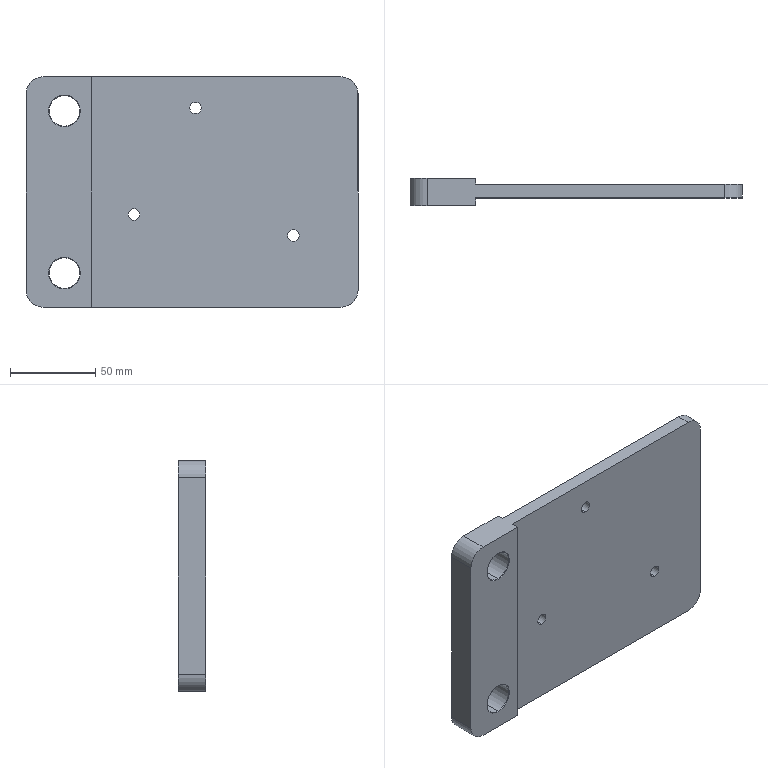Part | SolidWorks | features ICE 4, Chamfer 2, Fillet 1, FlatPattern 1, HoleWzd 1, SMBaseFlange 1, SheetMetal 1 | 1 solid | 39 faces | box 194.5 x 16 x 135 mm | volume 211709 mm3 | cylinder 16 | plane 11 | cone 10 | torus 2 | commonest cylinder face diameters 6.8 x6 18 x4 20 x4 83 x2
STEP:
#1=CARTESIAN_POINT('',(22.5,-0.3,11.));
#2=VERTEX_POINT('',#1);
#3=CARTESIAN_POINT('',(22.5,-0.3,29.));
#4=VERTEX_POINT('',#3);
#5=CARTESIAN_POINT('',(22.5,-0.3,20.));
#6=DIRECTION('',(0.,1.,0.));
#7=DIRECTION('',(0.,0.,-1.));
#8=AXIS2_PLACEMENT_3D('',#5,#6,#7);
#9=CIRCLE('',#8,9.);
#10=EDGE_CURVE('',#2,#4,#9,.T.);
#11=ORIENTED_EDGE('',*,*,#10,.F.);
#12=CARTESIAN_POINT('',(22.5,0.,10.7));
#13=VERTEX_POINT('',#12);
#14=CARTESIAN_POINT('',(22.5,-0.3,11.));
#15=DIRECTION('',(0.,0.7071,-0.7071));
#16=VECTOR('',#15,1000.);
#17=LINE('',#14,#16);
#18=EDGE_CURVE('',#2,#13,#17,.T.);
#19=ORIENTED_EDGE('',*,*,#18,.T.);
#20=CARTESIAN_POINT('',(22.5,0.,29.3));
#21=VERTEX_POINT('',#20);
#22=CARTESIAN_POINT('',(22.5,0.,20.));
#23=DIRECTION('',(0.,-1.,0.));
#24=DIRECTION('',(0.,0.,-1.));
#25=AXIS2_PLACEMENT_3D('',#22,#23,#24);
#26=CIRCLE('',#25,9.3);
#27=EDGE_CURVE('',#21,#13,#26,.T.);
#28=ORIENTED_EDGE('',*,*,#27,.F.);
#29=CARTESIAN_POINT('',(22.5,-0.3,29.));
#30=DIRECTION('',(0.,0.7071,0.7071));
#31=VECTOR('',#30,1000.);
#32=LINE('',#29,#31);
#33=EDGE_CURVE('',#4,#21,#32,.T.);
#34=ORIENTED_EDGE('',*,*,#33,.F.);
#35=EDGE_LOOP('',(#11,#19,#28,#34));
#36=FACE_OUTER_BOUND('',#35,.T.);
#37=CARTESIAN_POINT('',(22.5,-0.3,20.));
#38=DIRECTION('',(0.,1.,0.));
#39=DIRECTION('',(0.,0.,1.));
#40=AXIS2_PLACEMENT_3D('',#37,#38,#39);
#41=CONICAL_SURFACE('',#40,9.,0.7854);
#42=ADVANCED_FACE('',(#36),#41,.F.);
#43=CARTESIAN_POINT('',(22.5,-15.7,29.));
#44=VERTEX_POINT('',#43);
#45=CARTESIAN_POINT('',(22.5,-15.7,11.));
#46=VERTEX_POINT('',#45);
#47=CARTESIAN_POINT('',(22.5,-15.7,20.));
#48=DIRECTION('',(0.,-1.,0.));
#49=DIRECTION('',(0.,0.,-1.));
#50=AXIS2_PLACEMENT_3D('',#47,#48,#49);
#51=CIRCLE('',#50,9.);
#52=EDGE_CURVE('',#44,#46,#51,.T.);
#53=ORIENTED_EDGE('',*,*,#52,.F.);
#54=CARTESIAN_POINT('',(22.5,-16.,29.3));
#55=VERTEX_POINT('',#54);
#56=CARTESIAN_POINT('',(22.5,-16.,29.3));
#57=DIRECTION('',(0.,-0.7071,0.7071));
#58=VECTOR('',#57,1000.);
#59=LINE('',#56,#58);
#60=EDGE_CURVE('',#44,#55,#59,.T.);
#61=ORIENTED_EDGE('',*,*,#60,.T.);
#62=CARTESIAN_POINT('',(22.5,-16.,10.7));
#63=VERTEX_POINT('',#62);
#64=CARTESIAN_POINT('',(22.5,-16.,20.));
#65=DIRECTION('',(0.,1.,0.));
#66=DIRECTION('',(0.,0.,-1.));
#67=AXIS2_PLACEMENT_3D('',#64,#65,#66);
#68=CIRCLE('',#67,9.3);
#69=EDGE_CURVE('',#63,#55,#68,.T.);
#70=ORIENTED_EDGE('',*,*,#69,.F.);
#71=CARTESIAN_POINT('',(22.5,-16.,10.7));
#72=DIRECTION('',(0.,-0.7071,-0.7071));
#73=VECTOR('',#72,1000.);
#74=LINE('',#71,#73);
#75=EDGE_CURVE('',#46,#63,#74,.T.);
#76=ORIENTED_EDGE('',*,*,#75,.F.);
#77=EDGE_LOOP('',(#53,#61,#70,#76));
#78=FACE_OUTER_BOUND('',#77,.T.);
#79=CARTESIAN_POINT('',(22.5,-16.,20.));
#80=DIRECTION('',(0.,-1.,0.));
#81=DIRECTION('',(0.,0.,-1.));
#82=AXIS2_PLACEMENT_3D('',#79,#80,#81);
#83=CONICAL_SURFACE('',#82,9.3,0.7854);
#84=ADVANCED_FACE('',(#78),#83,.F.);
#85=CARTESIAN_POINT('',(22.5,-15.7,124.));
#86=VERTEX_POINT('',#85);
#87=CARTESIAN_POINT('',(22.5,-15.7,106.));
#88=VERTEX_POINT('',#87);
#89=CARTESIAN_POINT('',(22.5,-15.7,115.));
#90=DIRECTION('',(0.,-1.,0.));
#91=DIRECTION('',(0.,0.,-1.));
#92=AXIS2_PLACEMENT_3D('',#89,#90,#91);
#93=CIRCLE('',#92,9.);
#94=EDGE_CURVE('',#86,#88,#93,.T.);
#95=ORIENTED_EDGE('',*,*,#94,.F.);
#96=CARTESIAN_POINT('',(22.5,-16.,124.3));
#97=VERTEX_POINT('',#96);
#98=CARTESIAN_POINT('',(22.5,-16.,124.3));
#99=DIRECTION('',(0.,-0.7071,0.7071));
#100=VECTOR('',#99,1000.);
#101=LINE('',#98,#100);
#102=EDGE_CURVE('',#86,#97,#101,.T.);
#103=ORIENTED_EDGE('',*,*,#102,.T.);
#104=CARTESIAN_POINT('',(22.5,-16.,105.7));
#105=VERTEX_POINT('',#104);
#106=CARTESIAN_POINT('',(22.5,-16.,115.));
#107=DIRECTION('',(0.,1.,0.));
#108=DIRECTION('',(0.,0.,-1.));
#109=AXIS2_PLACEMENT_3D('',#106,#107,#108);
#110=CIRCLE('',#109,9.3);
#111=EDGE_CURVE('',#105,#97,#110,.T.);
#112=ORIENTED_EDGE('',*,*,#111,.F.);
#113=CARTESIAN_POINT('',(22.5,-16.,105.7));
#114=DIRECTION('',(0.,-0.7071,-0.7071));
#115=VECTOR('',#114,1000.);
#116=LINE('',#113,#115);
#117=EDGE_CURVE('',#88,#105,#116,.T.);
#118=ORIENTED_EDGE('',*,*,#117,.F.);
#119=EDGE_LOOP('',(#95,#103,#112,#118));
#120=FACE_OUTER_BOUND('',#119,.T.);
#121=CARTESIAN_POINT('',(22.5,-16.,115.));
#122=DIRECTION('',(0.,-1.,0.));
#123=DIRECTION('',(0.,0.,-1.));
#124=AXIS2_PLACEMENT_3D('',#121,#122,#123);
#125=CONICAL_SURFACE('',#124,9.3,0.7854);
#126=ADVANCED_FACE('',(#120),#125,.F.);
#127=CARTESIAN_POINT('',(22.5,-0.3,106.));
#128=VERTEX_POINT('',#127);
#129=CARTESIAN_POINT('',(22.5,-0.3,124.));
#130=VERTEX_POINT('',#129);
#131=CARTESIAN_POINT('',(22.5,-0.3,115.));
#132=DIRECTION('',(0.,1.,0.));
#133=DIRECTION('',(0.,0.,-1.));
#134=AXIS2_PLACEMENT_3D('',#131,#132,#133);
#135=CIRCLE('',#134,9.);
#136=EDGE_CURVE('',#128,#130,#135,.T.);
#137=ORIENTED_EDGE('',*,*,#136,.F.);
#138=CARTESIAN_POINT('',(22.5,0.,105.7));
#139=VERTEX_POINT('',#138);
#140=CARTESIAN_POINT('',(22.5,-0.3,106.));
#141=DIRECTION('',(0.,0.7071,-0.7071));
#142=VECTOR('',#141,1000.);
#143=LINE('',#140,#142);
#144=EDGE_CURVE('',#128,#139,#143,.T.);
#145=ORIENTED_EDGE('',*,*,#144,.T.);
#146=CARTESIAN_POINT('',(22.5,0.,124.3));
#147=VERTEX_POINT('',#146);
#148=CARTESIAN_POINT('',(22.5,0.,115.));
#149=DIRECTION('',(0.,-1.,0.));
#150=DIRECTION('',(0.,0.,-1.));
#151=AXIS2_PLACEMENT_3D('',#148,#149,#150);
#152=CIRCLE('',#151,9.3);
#153=EDGE_CURVE('',#147,#139,#152,.T.);
#154=ORIENTED_EDGE('',*,*,#153,.F.);
#155=CARTESIAN_POINT('',(22.5,-0.3,124.));
#156=DIRECTION('',(0.,0.7071,0.7071));
#157=VECTOR('',#156,1000.);
#158=LINE('',#155,#157);
#159=EDGE_CURVE('',#130,#147,#158,.T.);
#160=ORIENTED_EDGE('',*,*,#159,.F.);
#161=EDGE_LOOP('',(#137,#145,#154,#160));
#162=FACE_OUTER_BOUND('',#161,.T.);
#163=CARTESIAN_POINT('',(22.5,-0.3,115.));
#164=DIRECTION('',(0.,1.,0.));
#165=DIRECTION('',(0.,0.,1.));
#166=AXIS2_PLACEMENT_3D('',#163,#164,#165);
#167=CONICAL_SURFACE('',#166,9.,0.7854);
#168=ADVANCED_FACE('',(#162),#167,.F.);
#169=CARTESIAN_POINT('',(112.5,-4.5,26.));
#170=VERTEX_POINT('',#169);
#171=CARTESIAN_POINT('',(112.5,-4.5,109.));
#172=VERTEX_POINT('',#171);
#173=CARTESIAN_POINT('',(112.5,-4.5,67.5));
#174=DIRECTION('',(0.,1.,0.));
#175=DIRECTION('',(0.,0.,1.));
#176=AXIS2_PLACEMENT_3D('',#173,#174,#175);
#177=CIRCLE('',#176,41.5);
#178=EDGE_CURVE('',#170,#172,#177,.T.);
#179=ORIENTED_EDGE('',*,*,#178,.F.);
#180=CARTESIAN_POINT('',(112.5,-3.5,25.));
#181=VERTEX_POINT('',#180);
#182=CARTESIAN_POINT('',(112.5,-4.5,26.));
#183=DIRECTION('',(0.,0.7071,-0.7071));
#184=VECTOR('',#183,1000.);
#185=LINE('',#182,#184);
#186=EDGE_CURVE('',#170,#181,#185,.T.);
#187=ORIENTED_EDGE('',*,*,#186,.T.);
#188=CARTESIAN_POINT('',(112.5,-3.5,110.));
#189=VERTEX_POINT('',#188);
#190=CARTESIAN_POINT('',(112.5,-3.5,67.5));
#191=DIRECTION('',(0.,-1.,0.));
#192=DIRECTION('',(0.,0.,1.));
#193=AXIS2_PLACEMENT_3D('',#190,#191,#192);
#194=CIRCLE('',#193,42.5);
#195=EDGE_CURVE('',#189,#181,#194,.T.);
#196=ORIENTED_EDGE('',*,*,#195,.F.);
#197=CARTESIAN_POINT('',(112.5,-4.5,109.));
#198=DIRECTION('',(0.,0.7071,0.7071));
#199=VECTOR('',#198,1000.);
#200=LINE('',#197,#199);
#201=EDGE_CURVE('',#172,#189,#200,.T.);
#202=ORIENTED_EDGE('',*,*,#201,.F.);
#203=EDGE_LOOP('',(#179,#187,#196,#202));
#204=FACE_OUTER_BOUND('',#203,.T.);
#205=CARTESIAN_POINT('',(112.5,-4.5,67.5));
#206=DIRECTION('',(0.,1.,0.));
#207=DIRECTION('',(0.,0.,1.));
#208=AXIS2_PLACEMENT_3D('',#205,#206,#207);
#209=CONICAL_SURFACE('',#208,41.5,0.7854);
#210=ADVANCED_FACE('',(#204),#209,.F.);
#211=CARTESIAN_POINT('',(112.5,-9.,26.5));
#212=VERTEX_POINT('',#211);
#213=CARTESIAN_POINT('',(112.5,-9.,108.5));
#214=VERTEX_POINT('',#213);
#215=CARTESIAN_POINT('',(112.5,-9.,67.5));
#216=DIRECTION('',(0.,1.,0.));
#217=DIRECTION('',(0.,0.,1.));
#218=AXIS2_PLACEMENT_3D('',#215,#216,#217);
#219=CIRCLE('',#218,41.);
#220=EDGE_CURVE('',#212,#214,#219,.T.);
#221=ORIENTED_EDGE('',*,*,#220,.F.);
#222=CARTESIAN_POINT('',(112.5,-8.5,26.));
#223=VERTEX_POINT('',#222);
#224=CARTESIAN_POINT('',(112.5,-8.5,26.5));
#225=DIRECTION('',(1.,0.,0.));
#226=DIRECTION('',(0.,0.,-1.));
#227=AXIS2_PLACEMENT_3D('',#224,#225,#226);
#228=CIRCLE('',#227,0.5);
#229=EDGE_CURVE('',#212,#223,#228,.T.);
#230=ORIENTED_EDGE('',*,*,#229,.T.);
#231=CARTESIAN_POINT('',(112.5,-8.5,109.));
#232=VERTEX_POINT('',#231);
#233=CARTESIAN_POINT('',(112.5,-8.5,67.5));
#234=DIRECTION('',(0.,-1.,0.));
#235=DIRECTION('',(0.,0.,1.));
#236=AXIS2_PLACEMENT_3D('',#233,#234,#235);
#237=CIRCLE('',#236,41.5);
#238=EDGE_CURVE('',#232,#223,#237,.T.);
#239=ORIENTED_EDGE('',*,*,#238,.F.);
#240=CARTESIAN_POINT('',(112.5,-8.5,108.5));
#241=DIRECTION('',(-1.,0.,0.));
#242=DIRECTION('',(0.,0.,1.));
#243=AXIS2_PLACEMENT_3D('',#240,#241,#242);
#244=CIRCLE('',#243,0.5);
#245=EDGE_CURVE('',#214,#232,#244,.T.);
#246=ORIENTED_EDGE('',*,*,#245,.F.);
#247=EDGE_LOOP('',(#221,#230,#239,#246));
#248=FACE_OUTER_BOUND('',#247,.T.);
#249=CARTESIAN_POINT('',(112.5,-8.5,67.5));
#250=DIRECTION('',(0.,1.,0.));
#251=DIRECTION('',(0.,0.,1.));
#252=AXIS2_PLACEMENT_3D('',#249,#250,#251);
#253=TOROIDAL_SURFACE('',#252,41.,0.5);
#254=ADVANCED_FACE('',(#248),#253,.F.);
#255=CARTESIAN_POINT('',(63.238,-11.5,57.7));
#256=VERTEX_POINT('',#255);
#257=CARTESIAN_POINT('',(63.238,-11.5,50.9));
#258=VERTEX_POINT('',#257);
#259=CARTESIAN_POINT('',(63.238,-11.5,54.3));
#260=DIRECTION('',(0.,-1.,0.));
#261=DIRECTION('',(0.,0.,-1.));
#262=AXIS2_PLACEMENT_3D('',#259,#260,#261);
#263=CIRCLE('',#262,3.4);
#264=EDGE_CURVE('',#256,#258,#263,.T.);
#265=ORIENTED_EDGE('',*,*,#264,.T.);
#266=CARTESIAN_POINT('',(63.238,-3.5,50.9));
#267=VERTEX_POINT('',#266);
#268=CARTESIAN_POINT('',(63.238,-3.5,50.9));
#269=DIRECTION('',(0.,1.,0.));
#270=VECTOR('',#269,1000.);
#271=LINE('',#268,#270);
#272=EDGE_CURVE('',#258,#267,#271,.T.);
#273=ORIENTED_EDGE('',*,*,#272,.T.);
#274=CARTESIAN_POINT('',(63.238,-3.5,57.7));
#275=VERTEX_POINT('',#274);
#276=CARTESIAN_POINT('',(63.238,-3.5,54.3));
#277=DIRECTION('',(0.,1.,0.));
#278=DIRECTION('',(0.,0.,1.));
#279=AXIS2_PLACEMENT_3D('',#276,#277,#278);
#280=CIRCLE('',#279,3.4);
#281=EDGE_CURVE('',#267,#275,#280,.T.);
#282=ORIENTED_EDGE('',*,*,#281,.T.);
#283=CARTESIAN_POINT('',(63.238,-3.5,57.7));
#284=DIRECTION('',(0.,1.,0.));
#285=VECTOR('',#284,1000.);
#286=LINE('',#283,#285);
#287=EDGE_CURVE('',#256,#275,#286,.T.);
#288=ORIENTED_EDGE('',*,*,#287,.F.);
#289=EDGE_LOOP('',(#265,#273,#282,#288));
#290=FACE_OUTER_BOUND('',#289,.T.);
#291=CARTESIAN_POINT('',(63.238,-3.5,54.3));
#292=DIRECTION('',(0.,1.,0.));
#293=DIRECTION('',(0.,0.,1.));
#294=AXIS2_PLACEMENT_3D('',#291,#292,#293);
#295=CYLINDRICAL_SURFACE('',#294,3.4);
#296=ADVANCED_FACE('',(#290),#295,.F.);
#297=CARTESIAN_POINT('',(156.667,-11.5,45.4));
#298=VERTEX_POINT('',#297);
#299=CARTESIAN_POINT('',(156.667,-11.5,38.6));
#300=VERTEX_POINT('',#299);
#301=CARTESIAN_POINT('',(156.667,-11.5,42.));
#302=DIRECTION('',(0.,-1.,0.));
#303=DIRECTION('',(0.,0.,-1.));
#304=AXIS2_PLACEMENT_3D('',#301,#302,#303);
#305=CIRCLE('',#304,3.4);
#306=EDGE_CURVE('',#298,#300,#305,.T.);
#307=ORIENTED_EDGE('',*,*,#306,.T.);
#308=CARTESIAN_POINT('',(156.667,-3.5,38.6));
#309=VERTEX_POINT('',#308);
#310=CARTESIAN_POINT('',(156.667,-3.5,38.6));
#311=DIRECTION('',(0.,1.,0.));
#312=VECTOR('',#311,1000.);
#313=LINE('',#310,#312);
#314=EDGE_CURVE('',#300,#309,#313,.T.);
#315=ORIENTED_EDGE('',*,*,#314,.T.);
#316=CARTESIAN_POINT('',(156.667,-3.5,45.4));
#317=VERTEX_POINT('',#316);
#318=CARTESIAN_POINT('',(156.667,-3.5,42.));
#319=DIRECTION('',(0.,1.,0.));
#320=DIRECTION('',(0.,0.,1.));
#321=AXIS2_PLACEMENT_3D('',#318,#319,#320);
#322=CIRCLE('',#321,3.4);
#323=EDGE_CURVE('',#309,#317,#322,.T.);
#324=ORIENTED_EDGE('',*,*,#323,.T.);
#325=CARTESIAN_POINT('',(156.667,-3.5,45.4));
#326=DIRECTION('',(0.,1.,0.));
#327=VECTOR('',#326,1000.);
#328=LINE('',#325,#327);
#329=EDGE_CURVE('',#298,#317,#328,.T.);
#330=ORIENTED_EDGE('',*,*,#329,.F.);
#331=EDGE_LOOP('',(#307,#315,#324,#330));
#332=FACE_OUTER_BOUND('',#331,.T.);
#333=CARTESIAN_POINT('',(156.667,-3.5,42.));
#334=DIRECTION('',(0.,1.,0.));
#335=DIRECTION('',(0.,0.,1.));
#336=AXIS2_PLACEMENT_3D('',#333,#334,#335);
#337=CYLINDRICAL_SURFACE('',#336,3.4);
#338=ADVANCED_FACE('',(#332),#337,.F.);
#339=CARTESIAN_POINT('',(99.3,-11.5,120.162));
#340=VERTEX_POINT('',#339);
#341=CARTESIAN_POINT('',(99.3,-11.5,113.362));
#342=VERTEX_POINT('',#341);
#343=CARTESIAN_POINT('',(99.3,-11.5,116.762));
#344=DIRECTION('',(0.,-1.,0.));
#345=DIRECTION('',(0.,0.,-1.));
#346=AXIS2_PLACEMENT_3D('',#343,#344,#345);
#347=CIRCLE('',#346,3.4);
#348=EDGE_CURVE('',#340,#342,#347,.T.);
#349=ORIENTED_EDGE('',*,*,#348,.T.);
#350=CARTESIAN_POINT('',(99.3,-3.5,113.362));
#351=VERTEX_POINT('',#350);
#352=CARTESIAN_POINT('',(99.3,-3.5,113.362));
#353=DIRECTION('',(0.,1.,0.));
#354=VECTOR('',#353,1000.);
#355=LINE('',#352,#354);
#356=EDGE_CURVE('',#342,#351,#355,.T.);
#357=ORIENTED_EDGE('',*,*,#356,.T.);
#358=CARTESIAN_POINT('',(99.3,-3.5,120.162));
#359=VERTEX_POINT('',#358);
#360=CARTESIAN_POINT('',(99.3,-3.5,116.762));
#361=DIRECTION('',(0.,1.,0.));
#362=DIRECTION('',(0.,0.,1.));
#363=AXIS2_PLACEMENT_3D('',#360,#361,#362);
#364=CIRCLE('',#363,3.4);
#365=EDGE_CURVE('',#351,#359,#364,.T.);
#366=ORIENTED_EDGE('',*,*,#365,.T.);
#367=CARTESIAN_POINT('',(99.3,-3.5,120.162));
#368=DIRECTION('',(0.,1.,0.));
#369=VECTOR('',#368,1000.);
#370=LINE('',#367,#369);
#371=EDGE_CURVE('',#340,#359,#370,.T.);
#372=ORIENTED_EDGE('',*,*,#371,.F.);
#373=EDGE_LOOP('',(#349,#357,#366,#372));
#374=FACE_OUTER_BOUND('',#373,.T.);
#375=CARTESIAN_POINT('',(99.3,-3.5,116.762));
#376=DIRECTION('',(0.,1.,0.));
#377=DIRECTION('',(0.,0.,1.));
#378=AXIS2_PLACEMENT_3D('',#375,#376,#377);
#379=CYLINDRICAL_SURFACE('',#378,3.4);
#380=ADVANCED_FACE('',(#374),#379,.F.);
#381=ORIENTED_EDGE('',*,*,#238,.T.);
#382=CARTESIAN_POINT('',(112.5,-9.,26.));
#383=DIRECTION('',(0.,1.,0.));
#384=VECTOR('',#383,1000.);
#385=LINE('',#382,#384);
#386=EDGE_CURVE('',#223,#170,#385,.T.);
#387=ORIENTED_EDGE('',*,*,#386,.T.);
#388=ORIENTED_EDGE('',*,*,#178,.T.);
#389=CARTESIAN_POINT('',(112.5,-9.,109.));
#390=DIRECTION('',(0.,1.,0.));
#391=VECTOR('',#390,1000.);
#392=LINE('',#389,#391);
#393=EDGE_CURVE('',#232,#172,#392,.T.);
#394=ORIENTED_EDGE('',*,*,#393,.F.);
#395=EDGE_LOOP('',(#381,#387,#388,#394));
#396=FACE_OUTER_BOUND('',#395,.T.);
#397=CARTESIAN_POINT('',(112.5,-9.,67.5));
#398=DIRECTION('',(0.,1.,0.));
#399=DIRECTION('',(0.,0.,1.));
#400=AXIS2_PLACEMENT_3D('',#397,#398,#399);
#401=CYLINDRICAL_SURFACE('',#400,41.5);
#402=ADVANCED_FACE('',(#396),#401,.F.);
#403=ORIENTED_EDGE('',*,*,#94,.T.);
#404=CARTESIAN_POINT('',(22.5,-16.,106.));
#405=DIRECTION('',(0.,1.,0.));
#406=VECTOR('',#405,1000.);
#407=LINE('',#404,#406);
#408=EDGE_CURVE('',#88,#128,#407,.T.);
#409=ORIENTED_EDGE('',*,*,#408,.T.);
#410=ORIENTED_EDGE('',*,*,#136,.T.);
#411=CARTESIAN_POINT('',(22.5,-16.,124.));
#412=DIRECTION('',(0.,1.,0.));
#413=VECTOR('',#412,1000.);
#414=LINE('',#411,#413);
#415=EDGE_CURVE('',#86,#130,#414,.T.);
#416=ORIENTED_EDGE('',*,*,#415,.F.);
#417=EDGE_LOOP('',(#403,#409,#410,#416));
#418=FACE_OUTER_BOUND('',#417,.T.);
#419=CARTESIAN_POINT('',(22.5,-16.,115.));
#420=DIRECTION('',(0.,1.,0.));
#421=DIRECTION('',(0.,0.,1.));
#422=AXIS2_PLACEMENT_3D('',#419,#420,#421);
#423=CYLINDRICAL_SURFACE('',#422,9.);
#424=ADVANCED_FACE('',(#418),#423,.F.);
#425=ORIENTED_EDGE('',*,*,#52,.T.);
#426=CARTESIAN_POINT('',(22.5,-16.,11.));
#427=DIRECTION('',(0.,1.,0.));
#428=VECTOR('',#427,1000.);
#429=LINE('',#426,#428);
#430=EDGE_CURVE('',#46,#2,#429,.T.);
#431=ORIENTED_EDGE('',*,*,#430,.T.);
#432=ORIENTED_EDGE('',*,*,#10,.T.);
#433=CARTESIAN_POINT('',(22.5,-16.,29.));
#434=DIRECTION('',(0.,1.,0.));
#435=VECTOR('',#434,1000.);
#436=LINE('',#433,#435);
#437=EDGE_CURVE('',#44,#4,#436,.T.);
#438=ORIENTED_EDGE('',*,*,#437,.F.);
#439=EDGE_LOOP('',(#425,#431,#432,#438));
#440=FACE_OUTER_BOUND('',#439,.T.);
#441=CARTESIAN_POINT('',(22.5,-16.,20.));
#442=DIRECTION('',(0.,1.,0.));
#443=DIRECTION('',(0.,0.,1.));
#444=AXIS2_PLACEMENT_3D('',#441,#442,#443);
#445=CYLINDRICAL_SURFACE('',#444,9.);
#446=ADVANCED_FACE('',(#440),#445,.F.);
#447=CARTESIAN_POINT('',(194.5,-11.5,10.));
#448=VERTEX_POINT('',#447);
#449=CARTESIAN_POINT('',(194.5,-3.5,10.));
#450=VERTEX_POINT('',#449);
#451=CARTESIAN_POINT('',(194.5,-16.,10.));
#452=DIRECTION('',(0.,1.,0.));
#453=VECTOR('',#452,1000.);
#454=LINE('',#451,#453);
#455=EDGE_CURVE('',#448,#450,#454,.T.);
#456=ORIENTED_EDGE('',*,*,#455,.F.);
#457=CARTESIAN_POINT('',(184.5,-11.5,0.));
#458=VERTEX_POINT('',#457);
#459=CARTESIAN_POINT('',(184.5,-11.5,10.));
#460=DIRECTION('',(0.,1.,0.));
#461=DIRECTION('',(0.,0.,-1.));
#462=AXIS2_PLACEMENT_3D('',#459,#460,#461);
#463=CIRCLE('',#462,10.);
#464=EDGE_CURVE('',#448,#458,#463,.T.);
#465=ORIENTED_EDGE('',*,*,#464,.T.);
#466=CARTESIAN_POINT('',(184.5,-3.5,0.));
#467=VERTEX_POINT('',#466);
#468=CARTESIAN_POINT('',(184.5,-16.,0.));
#469=DIRECTION('',(0.,1.,0.));
#470=VECTOR('',#469,1000.);
#471=LINE('',#468,#470);
#472=EDGE_CURVE('',#458,#467,#471,.T.);
#473=ORIENTED_EDGE('',*,*,#472,.T.);
#474=CARTESIAN_POINT('',(184.5,-3.5,10.));
#475=DIRECTION('',(0.,-1.,0.));
#476=DIRECTION('',(0.,0.,1.));
#477=AXIS2_PLACEMENT_3D('',#474,#475,#476);
#478=CIRCLE('',#477,10.);
#479=EDGE_CURVE('',#467,#450,#478,.T.);
#480=ORIENTED_EDGE('',*,*,#479,.T.);
#481=EDGE_LOOP('',(#456,#465,#473,#480));
#482=FACE_OUTER_BOUND('',#481,.T.);
#483=CARTESIAN_POINT('',(184.5,-16.,10.));
#484=DIRECTION('',(0.,1.,0.));
#485=DIRECTION('',(0.,0.,1.));
#486=AXIS2_PLACEMENT_3D('',#483,#484,#485);
#487=CYLINDRICAL_SURFACE('',#486,10.);
#488=ADVANCED_FACE('',(#482),#487,.T.);
#489=CARTESIAN_POINT('',(194.5,-11.5,125.));
#490=VERTEX_POINT('',#489);
#491=CARTESIAN_POINT('',(194.5,-3.5,125.));
#492=VERTEX_POINT('',#491);
#493=CARTESIAN_POINT('',(194.5,-16.,125.));
#494=DIRECTION('',(0.,1.,0.));
#495=VECTOR('',#494,1000.);
#496=LINE('',#493,#495);
#497=EDGE_CURVE('',#490,#492,#496,.T.);
#498=ORIENTED_EDGE('',*,*,#497,.F.);
#499=CARTESIAN_POINT('',(194.5,-11.5,135.));
#500=DIRECTION('',(0.,0.,1.));
#501=VECTOR('',#500,1000.);
#502=LINE('',#499,#501);
#503=EDGE_CURVE('',#448,#490,#502,.T.);
#504=ORIENTED_EDGE('',*,*,#503,.F.);
#505=ORIENTED_EDGE('',*,*,#455,.T.);
#506=CARTESIAN_POINT('',(194.5,-3.5,0.));
#507=DIRECTION('',(0.,0.,-1.));
#508=VECTOR('',#507,1000.);
#509=LINE('',#506,#508);
#510=EDGE_CURVE('',#492,#450,#509,.T.);
#511=ORIENTED_EDGE('',*,*,#510,.F.);
#512=EDGE_LOOP('',(#498,#504,#505,#511));
#513=FACE_OUTER_BOUND('',#512,.T.);
#514=CARTESIAN_POINT('',(194.5,-16.,10.));
#515=DIRECTION('',(1.,0.,0.));
#516=DIRECTION('',(0.,0.,-1.));
#517=AXIS2_PLACEMENT_3D('',#514,#515,#516);
#518=PLANE('',#517);
#519=ADVANCED_FACE('',(#513),#518,.T.);
#520=CARTESIAN_POINT('',(184.5,-11.5,135.));
#521=VERTEX_POINT('',#520);
#522=CARTESIAN_POINT('',(184.5,-3.5,135.));
#523=VERTEX_POINT('',#522);
#524=CARTESIAN_POINT('',(184.5,-16.,135.));
#525=DIRECTION('',(0.,1.,0.));
#526=VECTOR('',#525,1000.);
#527=LINE('',#524,#526);
#528=EDGE_CURVE('',#521,#523,#527,.T.);
#529=ORIENTED_EDGE('',*,*,#528,.F.);
#530=CARTESIAN_POINT('',(184.5,-11.5,125.));
#531=DIRECTION('',(0.,1.,0.));
#532=DIRECTION('',(0.,0.,-1.));
#533=AXIS2_PLACEMENT_3D('',#530,#531,#532);
#534=CIRCLE('',#533,10.);
#535=EDGE_CURVE('',#521,#490,#534,.T.);
#536=ORIENTED_EDGE('',*,*,#535,.T.);
#537=ORIENTED_EDGE('',*,*,#497,.T.);
#538=CARTESIAN_POINT('',(184.5,-3.5,125.));
#539=DIRECTION('',(0.,-1.,0.));
#540=DIRECTION('',(0.,0.,1.));
#541=AXIS2_PLACEMENT_3D('',#538,#539,#540);
#542=CIRCLE('',#541,10.);
#543=EDGE_CURVE('',#492,#523,#542,.T.);
#544=ORIENTED_EDGE('',*,*,#543,.T.);
#545=EDGE_LOOP('',(#529,#536,#537,#544));
#546=FACE_OUTER_BOUND('',#545,.T.);
#547=CARTESIAN_POINT('',(184.5,-16.,125.));
#548=DIRECTION('',(0.,1.,0.));
#549=DIRECTION('',(0.,0.,1.));
#550=AXIS2_PLACEMENT_3D('',#547,#548,#549);
#551=CYLINDRICAL_SURFACE('',#550,10.);
#552=ADVANCED_FACE('',(#546),#551,.T.);
#553=CARTESIAN_POINT('',(38.5,-11.5,135.));
#554=VERTEX_POINT('',#553);
#555=CARTESIAN_POINT('',(38.5,-16.,135.));
#556=VERTEX_POINT('',#555);
#557=CARTESIAN_POINT('',(38.5,-11.5,135.));
#558=DIRECTION('',(0.,-1.,0.));
#559=VECTOR('',#558,1000.);
#560=LINE('',#557,#559);
#561=EDGE_CURVE('',#554,#556,#560,.T.);
#562=ORIENTED_EDGE('',*,*,#561,.F.);
#563=CARTESIAN_POINT('',(38.5,-11.5,135.));
#564=DIRECTION('',(-1.,0.,0.));
#565=VECTOR('',#564,1000.);
#566=LINE('',#563,#565);
#567=EDGE_CURVE('',#521,#554,#566,.T.);
#568=ORIENTED_EDGE('',*,*,#567,.F.);
#569=ORIENTED_EDGE('',*,*,#528,.T.);
#570=CARTESIAN_POINT('',(38.5,-3.5,135.));
#571=VERTEX_POINT('',#570);
#572=CARTESIAN_POINT('',(38.5,-3.5,135.));
#573=DIRECTION('',(1.,0.,0.));
#574=VECTOR('',#573,1000.);
#575=LINE('',#572,#574);
#576=EDGE_CURVE('',#571,#523,#575,.T.);
#577=ORIENTED_EDGE('',*,*,#576,.F.);
#578=CARTESIAN_POINT('',(38.5,0.,135.));
#579=VERTEX_POINT('',#578);
#580=CARTESIAN_POINT('',(38.5,-3.5,135.));
#581=DIRECTION('',(0.,1.,0.));
#582=VECTOR('',#581,1000.);
#583=LINE('',#580,#582);
#584=EDGE_CURVE('',#571,#579,#583,.T.);
#585=ORIENTED_EDGE('',*,*,#584,.T.);
#586=CARTESIAN_POINT('',(10.,0.,135.));
#587=VERTEX_POINT('',#586);
#588=CARTESIAN_POINT('',(10.,0.,135.));
#589=DIRECTION('',(1.,0.,0.));
#590=VECTOR('',#589,1000.);
#591=LINE('',#588,#590);
#592=EDGE_CURVE('',#587,#579,#591,.T.);
#593=ORIENTED_EDGE('',*,*,#592,.F.);
#594=CARTESIAN_POINT('',(10.,-16.,135.));
#595=VERTEX_POINT('',#594);
#596=CARTESIAN_POINT('',(10.,-16.,135.));
#597=DIRECTION('',(0.,1.,0.));
#598=VECTOR('',#597,1000.);
#599=LINE('',#596,#598);
#600=EDGE_CURVE('',#595,#587,#599,.T.);
#601=ORIENTED_EDGE('',*,*,#600,.F.);
#602=CARTESIAN_POINT('',(10.,-16.,135.));
#603=DIRECTION('',(1.,0.,0.));
#604=VECTOR('',#603,1000.);
#605=LINE('',#602,#604);
#606=EDGE_CURVE('',#595,#556,#605,.T.);
#607=ORIENTED_EDGE('',*,*,#606,.T.);
#608=EDGE_LOOP('',(#562,#568,#569,#577,#585,#593,#601,#607));
#609=FACE_OUTER_BOUND('',#608,.T.);
#610=CARTESIAN_POINT('',(10.,-16.,135.));
#611=DIRECTION('',(0.,0.,1.));
#612=DIRECTION('',(1.,0.,0.));
#613=AXIS2_PLACEMENT_3D('',#610,#611,#612);
#614=PLANE('',#613);
#615=ADVANCED_FACE('',(#609),#614,.T.);
#616=CARTESIAN_POINT('',(0.,0.,125.));
#617=VERTEX_POINT('',#616);
#618=CARTESIAN_POINT('',(10.,0.,125.));
#619=DIRECTION('',(0.,1.,0.));
#620=DIRECTION('',(0.,0.,1.));
#621=AXIS2_PLACEMENT_3D('',#618,#619,#620);
#622=CIRCLE('',#621,10.);
#623=EDGE_CURVE('',#617,#587,#622,.T.);
#624=ORIENTED_EDGE('',*,*,#623,.F.);
#625=CARTESIAN_POINT('',(0.,-16.,125.));
#626=VERTEX_POINT('',#625);
#627=CARTESIAN_POINT('',(0.,-16.,125.));
#628=DIRECTION('',(0.,1.,0.));
#629=VECTOR('',#628,1000.);
#630=LINE('',#627,#629);
#631=EDGE_CURVE('',#626,#617,#630,.T.);
#632=ORIENTED_EDGE('',*,*,#631,.F.);
#633=CARTESIAN_POINT('',(10.,-16.,125.));
#634=DIRECTION('',(0.,1.,0.));
#635=DIRECTION('',(0.,0.,1.));
#636=AXIS2_PLACEMENT_3D('',#633,#634,#635);
#637=CIRCLE('',#636,10.);
#638=EDGE_CURVE('',#626,#595,#637,.T.);
#639=ORIENTED_EDGE('',*,*,#638,.T.);
#640=ORIENTED_EDGE('',*,*,#600,.T.);
#641=EDGE_LOOP('',(#624,#632,#639,#640));
#642=FACE_OUTER_BOUND('',#641,.T.);
#643=CARTESIAN_POINT('',(10.,-16.,125.));
#644=DIRECTION('',(0.,1.,0.));
#645=DIRECTION('',(0.,0.,1.));
#646=AXIS2_PLACEMENT_3D('',#643,#644,#645);
#647=CYLINDRICAL_SURFACE('',#646,10.);
#648=ADVANCED_FACE('',(#642),#647,.T.);
#649=CARTESIAN_POINT('',(0.,0.,10.));
#650=VERTEX_POINT('',#649);
#651=CARTESIAN_POINT('',(0.,0.,10.));
#652=DIRECTION('',(0.,0.,1.));
#653=VECTOR('',#652,1000.);
#654=LINE('',#651,#653);
#655=EDGE_CURVE('',#650,#617,#654,.T.);
#656=ORIENTED_EDGE('',*,*,#655,.F.);
#657=CARTESIAN_POINT('',(0.,-16.,10.));
#658=VERTEX_POINT('',#657);
#659=CARTESIAN_POINT('',(0.,-16.,10.));
#660=DIRECTION('',(0.,1.,0.));
#661=VECTOR('',#660,1000.);
#662=LINE('',#659,#661);
#663=EDGE_CURVE('',#658,#650,#662,.T.);
#664=ORIENTED_EDGE('',*,*,#663,.F.);
#665=CARTESIAN_POINT('',(0.,-16.,10.));
#666=DIRECTION('',(0.,0.,1.));
#667=VECTOR('',#666,1000.);
#668=LINE('',#665,#667);
#669=EDGE_CURVE('',#658,#626,#668,.T.);
#670=ORIENTED_EDGE('',*,*,#669,.T.);
#671=ORIENTED_EDGE('',*,*,#631,.T.);
#672=EDGE_LOOP('',(#656,#664,#670,#671));
#673=FACE_OUTER_BOUND('',#672,.T.);
#674=CARTESIAN_POINT('',(0.,-16.,10.));
#675=DIRECTION('',(-1.,0.,0.));
#676=DIRECTION('',(0.,0.,1.));
#677=AXIS2_PLACEMENT_3D('',#674,#675,#676);
#678=PLANE('',#677);
#679=ADVANCED_FACE('',(#673),#678,.T.);
#680=CARTESIAN_POINT('',(10.,0.,0.));
#681=VERTEX_POINT('',#680);
#682=CARTESIAN_POINT('',(10.,0.,10.));
#683=DIRECTION('',(0.,1.,0.));
#684=DIRECTION('',(0.,0.,1.));
#685=AXIS2_PLACEMENT_3D('',#682,#683,#684);
#686=CIRCLE('',#685,10.);
#687=EDGE_CURVE('',#681,#650,#686,.T.);
#688=ORIENTED_EDGE('',*,*,#687,.F.);
#689=CARTESIAN_POINT('',(10.,-16.,0.));
#690=VERTEX_POINT('',#689);
#691=CARTESIAN_POINT('',(10.,-16.,0.));
#692=DIRECTION('',(0.,1.,0.));
#693=VECTOR('',#692,1000.);
#694=LINE('',#691,#693);
#695=EDGE_CURVE('',#690,#681,#694,.T.);
#696=ORIENTED_EDGE('',*,*,#695,.F.);
#697=CARTESIAN_POINT('',(10.,-16.,10.));
#698=DIRECTION('',(0.,1.,0.));
#699=DIRECTION('',(0.,0.,1.));
#700=AXIS2_PLACEMENT_3D('',#697,#698,#699);
#701=CIRCLE('',#700,10.);
#702=EDGE_CURVE('',#690,#658,#701,.T.);
#703=ORIENTED_EDGE('',*,*,#702,.T.);
#704=ORIENTED_EDGE('',*,*,#663,.T.);
#705=EDGE_LOOP('',(#688,#696,#703,#704));
#706=FACE_OUTER_BOUND('',#705,.T.);
#707=CARTESIAN_POINT('',(10.,-16.,10.));
#708=DIRECTION('',(0.,1.,0.));
#709=DIRECTION('',(0.,0.,1.));
#710=AXIS2_PLACEMENT_3D('',#707,#708,#709);
#711=CYLINDRICAL_SURFACE('',#710,10.);
#712=ADVANCED_FACE('',(#706),#711,.T.);
#713=CARTESIAN_POINT('',(38.5,-11.5,0.));
#714=VERTEX_POINT('',#713);
#715=CARTESIAN_POINT('',(38.5,-16.,0.));
#716=VERTEX_POINT('',#715);
#717=CARTESIAN_POINT('',(38.5,-11.5,0.));
#718=DIRECTION('',(0.,-1.,0.));
#719=VECTOR('',#718,1000.);
#720=LINE('',#717,#719);
#721=EDGE_CURVE('',#714,#716,#720,.T.);
#722=ORIENTED_EDGE('',*,*,#721,.T.);
#723=CARTESIAN_POINT('',(10.,-16.,0.));
#724=DIRECTION('',(-1.,0.,0.));
#725=VECTOR('',#724,1000.);
#726=LINE('',#723,#725);
#727=EDGE_CURVE('',#716,#690,#726,.T.);
#728=ORIENTED_EDGE('',*,*,#727,.T.);
#729=ORIENTED_EDGE('',*,*,#695,.T.);
#730=CARTESIAN_POINT('',(38.5,0.,0.));
#731=VERTEX_POINT('',#730);
#732=CARTESIAN_POINT('',(10.,0.,0.));
#733=DIRECTION('',(-1.,0.,0.));
#734=VECTOR('',#733,1000.);
#735=LINE('',#732,#734);
#736=EDGE_CURVE('',#731,#681,#735,.T.);
#737=ORIENTED_EDGE('',*,*,#736,.F.);
#738=CARTESIAN_POINT('',(38.5,-3.5,0.));
#739=VERTEX_POINT('',#738);
#740=CARTESIAN_POINT('',(38.5,-3.5,0.));
#741=DIRECTION('',(0.,1.,0.));
#742=VECTOR('',#741,1000.);
#743=LINE('',#740,#742);
#744=EDGE_CURVE('',#739,#731,#743,.T.);
#745=ORIENTED_EDGE('',*,*,#744,.F.);
#746=CARTESIAN_POINT('',(38.5,-3.5,0.));
#747=DIRECTION('',(-1.,0.,0.));
#748=VECTOR('',#747,1000.);
#749=LINE('',#746,#748);
#750=EDGE_CURVE('',#467,#739,#749,.T.);
#751=ORIENTED_EDGE('',*,*,#750,.F.);
#752=ORIENTED_EDGE('',*,*,#472,.F.);
#753=CARTESIAN_POINT('',(38.5,-11.5,0.));
#754=DIRECTION('',(1.,0.,0.));
#755=VECTOR('',#754,1000.);
#756=LINE('',#753,#755);
#757=EDGE_CURVE('',#714,#458,#756,.T.);
#758=ORIENTED_EDGE('',*,*,#757,.F.);
#759=EDGE_LOOP('',(#722,#728,#729,#737,#745,#751,#752,#758));
#760=FACE_OUTER_BOUND('',#759,.T.);
#761=CARTESIAN_POINT('',(10.,-16.,0.));
#762=DIRECTION('',(0.,0.,-1.));
#763=DIRECTION('',(-1.,0.,0.));
#764=AXIS2_PLACEMENT_3D('',#761,#762,#763);
#765=PLANE('',#764);
#766=ADVANCED_FACE('',(#760),#765,.T.);
#767=ORIENTED_EDGE('',*,*,#111,.T.);
#768=CARTESIAN_POINT('',(22.5,-16.,115.));
#769=DIRECTION('',(0.,1.,0.));
#770=DIRECTION('',(0.,0.,-1.));
#771=AXIS2_PLACEMENT_3D('',#768,#769,#770);
#772=CIRCLE('',#771,9.3);
#773=EDGE_CURVE('',#97,#105,#772,.T.);
#774=ORIENTED_EDGE('',*,*,#773,.T.);
#775=EDGE_LOOP('',(#767,#774));
#776=FACE_BOUND('',#775,.T.);
#777=ORIENTED_EDGE('',*,*,#69,.T.);
#778=CARTESIAN_POINT('',(22.5,-16.,20.));
#779=DIRECTION('',(0.,1.,0.));
#780=DIRECTION('',(0.,0.,-1.));
#781=AXIS2_PLACEMENT_3D('',#778,#779,#780);
#782=CIRCLE('',#781,9.3);
#783=EDGE_CURVE('',#55,#63,#782,.T.);
#784=ORIENTED_EDGE('',*,*,#783,.T.);
#785=EDGE_LOOP('',(#777,#784));
#786=FACE_BOUND('',#785,.T.);
#787=CARTESIAN_POINT('',(38.5,-16.,135.));
#788=DIRECTION('',(0.,0.,-1.));
#789=VECTOR('',#788,1000.);
#790=LINE('',#787,#789);
#791=EDGE_CURVE('',#556,#716,#790,.T.);
#792=ORIENTED_EDGE('',*,*,#791,.F.);
#793=ORIENTED_EDGE('',*,*,#606,.F.);
#794=ORIENTED_EDGE('',*,*,#638,.F.);
#795=ORIENTED_EDGE('',*,*,#669,.F.);
#796=ORIENTED_EDGE('',*,*,#702,.F.);
#797=ORIENTED_EDGE('',*,*,#727,.F.);
#798=EDGE_LOOP('',(#792,#793,#794,#795,#796,#797));
#799=FACE_OUTER_BOUND('',#798,.T.);
#800=CARTESIAN_POINT('',(184.5,-16.,10.));
#801=DIRECTION('',(0.,-1.,0.));
#802=DIRECTION('',(0.,0.,-1.));
#803=AXIS2_PLACEMENT_3D('',#800,#801,#802);
#804=PLANE('',#803);
#805=ADVANCED_FACE('',(#776,#786,#799),#804,.T.);
#806=ORIENTED_EDGE('',*,*,#153,.T.);
#807=CARTESIAN_POINT('',(22.5,0.,115.));
#808=DIRECTION('',(0.,-1.,0.));
#809=DIRECTION('',(0.,0.,-1.));
#810=AXIS2_PLACEMENT_3D('',#807,#808,#809);
#811=CIRCLE('',#810,9.3);
#812=EDGE_CURVE('',#139,#147,#811,.T.);
#813=ORIENTED_EDGE('',*,*,#812,.T.);
#814=EDGE_LOOP('',(#806,#813));
#815=FACE_BOUND('',#814,.T.);
#816=ORIENTED_EDGE('',*,*,#27,.T.);
#817=CARTESIAN_POINT('',(22.5,0.,20.));
#818=DIRECTION('',(0.,-1.,0.));
#819=DIRECTION('',(0.,0.,-1.));
#820=AXIS2_PLACEMENT_3D('',#817,#818,#819);
#821=CIRCLE('',#820,9.3);
#822=EDGE_CURVE('',#13,#21,#821,.T.);
#823=ORIENTED_EDGE('',*,*,#822,.T.);
#824=EDGE_LOOP('',(#816,#823));
#825=FACE_BOUND('',#824,.T.);
#826=ORIENTED_EDGE('',*,*,#592,.T.);
#827=CARTESIAN_POINT('',(38.5,0.,0.));
#828=DIRECTION('',(0.,0.,1.));
#829=VECTOR('',#828,1000.);
#830=LINE('',#827,#829);
#831=EDGE_CURVE('',#731,#579,#830,.T.);
#832=ORIENTED_EDGE('',*,*,#831,.F.);
#833=ORIENTED_EDGE('',*,*,#736,.T.);
#834=ORIENTED_EDGE('',*,*,#687,.T.);
#835=ORIENTED_EDGE('',*,*,#655,.T.);
#836=ORIENTED_EDGE('',*,*,#623,.T.);
#837=EDGE_LOOP('',(#826,#832,#833,#834,#835,#836));
#838=FACE_OUTER_BOUND('',#837,.T.);
#839=CARTESIAN_POINT('',(184.5,0.,10.));
#840=DIRECTION('',(0.,-1.,0.));
#841=DIRECTION('',(0.,0.,-1.));
#842=AXIS2_PLACEMENT_3D('',#839,#840,#841);
#843=PLANE('',#842);
#844=ADVANCED_FACE('',(#815,#825,#838),#843,.F.);
#845=ORIENTED_EDGE('',*,*,#430,.F.);
#846=CARTESIAN_POINT('',(22.5,-15.7,20.));
#847=DIRECTION('',(0.,-1.,0.));
#848=DIRECTION('',(0.,0.,-1.));
#849=AXIS2_PLACEMENT_3D('',#846,#847,#848);
#850=CIRCLE('',#849,9.);
#851=EDGE_CURVE('',#46,#44,#850,.T.);
#852=ORIENTED_EDGE('',*,*,#851,.T.);
#853=ORIENTED_EDGE('',*,*,#437,.T.);
#854=CARTESIAN_POINT('',(22.5,-0.3,20.));
#855=DIRECTION('',(0.,1.,0.));
#856=DIRECTION('',(0.,0.,-1.));
#857=AXIS2_PLACEMENT_3D('',#854,#855,#856);
#858=CIRCLE('',#857,9.);
#859=EDGE_CURVE('',#4,#2,#858,.T.);
#860=ORIENTED_EDGE('',*,*,#859,.T.);
#861=EDGE_LOOP('',(#845,#852,#853,#860));
#862=FACE_OUTER_BOUND('',#861,.T.);
#863=CARTESIAN_POINT('',(22.5,-16.,20.));
#864=DIRECTION('',(0.,1.,0.));
#865=DIRECTION('',(0.,0.,1.));
#866=AXIS2_PLACEMENT_3D('',#863,#864,#865);
#867=CYLINDRICAL_SURFACE('',#866,9.);
#868=ADVANCED_FACE('',(#862),#867,.F.);
#869=ORIENTED_EDGE('',*,*,#408,.F.);
#870=CARTESIAN_POINT('',(22.5,-15.7,115.));
#871=DIRECTION('',(0.,-1.,0.));
#872=DIRECTION('',(0.,0.,-1.));
#873=AXIS2_PLACEMENT_3D('',#870,#871,#872);
#874=CIRCLE('',#873,9.);
#875=EDGE_CURVE('',#88,#86,#874,.T.);
#876=ORIENTED_EDGE('',*,*,#875,.T.);
#877=ORIENTED_EDGE('',*,*,#415,.T.);
#878=CARTESIAN_POINT('',(22.5,-0.3,115.));
#879=DIRECTION('',(0.,1.,0.));
#880=DIRECTION('',(0.,0.,-1.));
#881=AXIS2_PLACEMENT_3D('',#878,#879,#880);
#882=CIRCLE('',#881,9.);
#883=EDGE_CURVE('',#130,#128,#882,.T.);
#884=ORIENTED_EDGE('',*,*,#883,.T.);
#885=EDGE_LOOP('',(#869,#876,#877,#884));
#886=FACE_OUTER_BOUND('',#885,.T.);
#887=CARTESIAN_POINT('',(22.5,-16.,115.));
#888=DIRECTION('',(0.,1.,0.));
#889=DIRECTION('',(0.,0.,1.));
#890=AXIS2_PLACEMENT_3D('',#887,#888,#889);
#891=CYLINDRICAL_SURFACE('',#890,9.);
#892=ADVANCED_FACE('',(#886),#891,.F.);
#893=ORIENTED_EDGE('',*,*,#831,.T.);
#894=ORIENTED_EDGE('',*,*,#584,.F.);
#895=CARTESIAN_POINT('',(38.5,-3.5,0.));
#896=DIRECTION('',(0.,0.,1.));
#897=VECTOR('',#896,1000.);
#898=LINE('',#895,#897);
#899=EDGE_CURVE('',#739,#571,#898,.T.);
#900=ORIENTED_EDGE('',*,*,#899,.F.);
#901=ORIENTED_EDGE('',*,*,#744,.T.);
#902=EDGE_LOOP('',(#893,#894,#900,#901));
#903=FACE_OUTER_BOUND('',#902,.T.);
#904=CARTESIAN_POINT('',(38.5,-3.5,0.));
#905=DIRECTION('',(-1.,0.,0.));
#906=DIRECTION('',(0.,0.,1.));
#907=AXIS2_PLACEMENT_3D('',#904,#905,#906);
#908=PLANE('',#907);
#909=ADVANCED_FACE('',(#903),#908,.F.);
#910=ORIENTED_EDGE('',*,*,#195,.T.);
#911=CARTESIAN_POINT('',(112.5,-3.5,67.5));
#912=DIRECTION('',(0.,-1.,0.));
#913=DIRECTION('',(0.,0.,1.));
#914=AXIS2_PLACEMENT_3D('',#911,#912,#913);
#915=CIRCLE('',#914,42.5);
#916=EDGE_CURVE('',#181,#189,#915,.T.);
#917=ORIENTED_EDGE('',*,*,#916,.T.);
#918=EDGE_LOOP('',(#910,#917));
#919=FACE_BOUND('',#918,.T.);
#920=CARTESIAN_POINT('',(63.238,-3.5,54.3));
#921=DIRECTION('',(0.,1.,0.));
#922=DIRECTION('',(0.,0.,1.));
#923=AXIS2_PLACEMENT_3D('',#920,#921,#922);
#924=CIRCLE('',#923,3.4);
#925=EDGE_CURVE('',#275,#267,#924,.T.);
#926=ORIENTED_EDGE('',*,*,#925,.F.);
#927=ORIENTED_EDGE('',*,*,#281,.F.);
#928=EDGE_LOOP('',(#926,#927));
#929=FACE_BOUND('',#928,.T.);
#930=CARTESIAN_POINT('',(156.667,-3.5,42.));
#931=DIRECTION('',(0.,1.,0.));
#932=DIRECTION('',(0.,0.,1.));
#933=AXIS2_PLACEMENT_3D('',#930,#931,#932);
#934=CIRCLE('',#933,3.4);
#935=EDGE_CURVE('',#317,#309,#934,.T.);
#936=ORIENTED_EDGE('',*,*,#935,.F.);
#937=ORIENTED_EDGE('',*,*,#323,.F.);
#938=EDGE_LOOP('',(#936,#937));
#939=FACE_BOUND('',#938,.T.);
#940=CARTESIAN_POINT('',(99.3,-3.5,116.762));
#941=DIRECTION('',(0.,1.,0.));
#942=DIRECTION('',(0.,0.,1.));
#943=AXIS2_PLACEMENT_3D('',#940,#941,#942);
#944=CIRCLE('',#943,3.4);
#945=EDGE_CURVE('',#359,#351,#944,.T.);
#946=ORIENTED_EDGE('',*,*,#945,.F.);
#947=ORIENTED_EDGE('',*,*,#365,.F.);
#948=EDGE_LOOP('',(#946,#947));
#949=FACE_BOUND('',#948,.T.);
#950=ORIENTED_EDGE('',*,*,#750,.T.);
#951=ORIENTED_EDGE('',*,*,#899,.T.);
#952=ORIENTED_EDGE('',*,*,#576,.T.);
#953=ORIENTED_EDGE('',*,*,#543,.F.);
#954=ORIENTED_EDGE('',*,*,#510,.T.);
#955=ORIENTED_EDGE('',*,*,#479,.F.);
#956=EDGE_LOOP('',(#950,#951,#952,#953,#954,#955));
#957=FACE_OUTER_BOUND('',#956,.T.);
#958=CARTESIAN_POINT('',(0.,-3.5,0.));
#959=DIRECTION('',(0.,1.,0.));
#960=DIRECTION('',(0.,0.,1.));
#961=AXIS2_PLACEMENT_3D('',#958,#959,#960);
#962=PLANE('',#961);
#963=ADVANCED_FACE('',(#919,#929,#939,#949,#957),#962,.T.);
#964=ORIENTED_EDGE('',*,*,#791,.T.);
#965=ORIENTED_EDGE('',*,*,#721,.F.);
#966=CARTESIAN_POINT('',(38.5,-11.5,135.));
#967=DIRECTION('',(0.,0.,-1.));
#968=VECTOR('',#967,1000.);
#969=LINE('',#966,#968);
#970=EDGE_CURVE('',#554,#714,#969,.T.);
#971=ORIENTED_EDGE('',*,*,#970,.F.);
#972=ORIENTED_EDGE('',*,*,#561,.T.);
#973=EDGE_LOOP('',(#964,#965,#971,#972));
#974=FACE_OUTER_BOUND('',#973,.T.);
#975=CARTESIAN_POINT('',(38.5,-11.5,135.));
#976=DIRECTION('',(-1.,0.,0.));
#977=DIRECTION('',(0.,0.,1.));
#978=AXIS2_PLACEMENT_3D('',#975,#976,#977);
#979=PLANE('',#978);
#980=ADVANCED_FACE('',(#974),#979,.F.);
#981=ORIENTED_EDGE('',*,*,#264,.F.);
#982=CARTESIAN_POINT('',(63.238,-11.5,54.3));
#983=DIRECTION('',(0.,-1.,0.));
#984=DIRECTION('',(0.,0.,-1.));
#985=AXIS2_PLACEMENT_3D('',#982,#983,#984);
#986=CIRCLE('',#985,3.4);
#987=EDGE_CURVE('',#258,#256,#986,.T.);
#988=ORIENTED_EDGE('',*,*,#987,.F.);
#989=EDGE_LOOP('',(#981,#988));
#990=FACE_BOUND('',#989,.T.);
#991=ORIENTED_EDGE('',*,*,#306,.F.);
#992=CARTESIAN_POINT('',(156.667,-11.5,42.));
#993=DIRECTION('',(0.,-1.,0.));
#994=DIRECTION('',(0.,0.,-1.));
#995=AXIS2_PLACEMENT_3D('',#992,#993,#994);
#996=CIRCLE('',#995,3.4);
#997=EDGE_CURVE('',#300,#298,#996,.T.);
#998=ORIENTED_EDGE('',*,*,#997,.F.);
#999=EDGE_LOOP('',(#991,#998));
#1000=FACE_BOUND('',#999,.T.);
#1001=ORIENTED_EDGE('',*,*,#348,.F.);
#1002=CARTESIAN_POINT('',(99.3,-11.5,116.762));
#1003=DIRECTION('',(0.,-1.,0.));
#1004=DIRECTION('',(0.,0.,-1.));
#1005=AXIS2_PLACEMENT_3D('',#1002,#1003,#1004);
#1006=CIRCLE('',#1005,3.4);
#1007=EDGE_CURVE('',#342,#340,#1006,.T.);
#1008=ORIENTED_EDGE('',*,*,#1007,.F.);
#1009=EDGE_LOOP('',(#1001,#1008));
#1010=FACE_BOUND('',#1009,.T.);
#1011=ORIENTED_EDGE('',*,*,#503,.T.);
#1012=ORIENTED_EDGE('',*,*,#535,.F.);
#1013=ORIENTED_EDGE('',*,*,#567,.T.);
#1014=ORIENTED_EDGE('',*,*,#970,.T.);
#1015=ORIENTED_EDGE('',*,*,#757,.T.);
#1016=ORIENTED_EDGE('',*,*,#464,.F.);
#1017=EDGE_LOOP('',(#1011,#1012,#1013,#1014,#1015,#1016));
#1018=FACE_OUTER_BOUND('',#1017,.T.);
#1019=CARTESIAN_POINT('',(0.,-11.5,0.));
#1020=DIRECTION('',(0.,-1.,0.));
#1021=DIRECTION('',(0.,0.,-1.));
#1022=AXIS2_PLACEMENT_3D('',#1019,#1020,#1021);
#1023=PLANE('',#1022);
#1024=ADVANCED_FACE('',(#990,#1000,#1010,#1018),#1023,.T.);
#1025=ORIENTED_EDGE('',*,*,#386,.F.);
#1026=CARTESIAN_POINT('',(112.5,-8.5,67.5));
#1027=DIRECTION('',(0.,-1.,0.));
#1028=DIRECTION('',(0.,0.,1.));
#1029=AXIS2_PLACEMENT_3D('',#1026,#1027,#1028);
#1030=CIRCLE('',#1029,41.5);
#1031=EDGE_CURVE('',#223,#232,#1030,.T.);
#1032=ORIENTED_EDGE('',*,*,#1031,.T.);
#1033=ORIENTED_EDGE('',*,*,#393,.T.);
#1034=CARTESIAN_POINT('',(112.5,-4.5,67.5));
#1035=DIRECTION('',(0.,1.,0.));
#1036=DIRECTION('',(0.,0.,1.));
#1037=AXIS2_PLACEMENT_3D('',#1034,#1035,#1036);
#1038=CIRCLE('',#1037,41.5);
#1039=EDGE_CURVE('',#172,#170,#1038,.T.);
#1040=ORIENTED_EDGE('',*,*,#1039,.T.);
#1041=EDGE_LOOP('',(#1025,#1032,#1033,#1040));
#1042=FACE_OUTER_BOUND('',#1041,.T.);
#1043=CARTESIAN_POINT('',(112.5,-9.,67.5));
#1044=DIRECTION('',(0.,1.,0.));
#1045=DIRECTION('',(0.,0.,1.));
#1046=AXIS2_PLACEMENT_3D('',#1043,#1044,#1045);
#1047=CYLINDRICAL_SURFACE('',#1046,41.5);
#1048=ADVANCED_FACE('',(#1042),#1047,.F.);
#1049=CARTESIAN_POINT('',(112.5,-9.,67.5));
#1050=DIRECTION('',(0.,1.,0.));
#1051=DIRECTION('',(0.,0.,1.));
#1052=AXIS2_PLACEMENT_3D('',#1049,#1050,#1051);
#1053=CIRCLE('',#1052,41.);
#1054=EDGE_CURVE('',#214,#212,#1053,.T.);
#1055=ORIENTED_EDGE('',*,*,#1054,.T.);
#1056=ORIENTED_EDGE('',*,*,#220,.T.);
#1057=EDGE_LOOP('',(#1055,#1056));
#1058=FACE_OUTER_BOUND('',#1057,.T.);
#1059=CARTESIAN_POINT('',(112.5,-9.,67.5));
#1060=DIRECTION('',(0.,1.,0.));
#1061=DIRECTION('',(0.,0.,1.));
#1062=AXIS2_PLACEMENT_3D('',#1059,#1060,#1061);
#1063=PLANE('',#1062);
#1064=ADVANCED_FACE('',(#1058),#1063,.T.);
#1065=ORIENTED_EDGE('',*,*,#356,.F.);
#1066=ORIENTED_EDGE('',*,*,#1007,.T.);
#1067=ORIENTED_EDGE('',*,*,#371,.T.);
#1068=ORIENTED_EDGE('',*,*,#945,.T.);
#1069=EDGE_LOOP('',(#1065,#1066,#1067,#1068));
#1070=FACE_OUTER_BOUND('',#1069,.T.);
#1071=CARTESIAN_POINT('',(99.3,-3.5,116.762));
#1072=DIRECTION('',(0.,1.,0.));
#1073=DIRECTION('',(0.,0.,1.));
#1074=AXIS2_PLACEMENT_3D('',#1071,#1072,#1073);
#1075=CYLINDRICAL_SURFACE('',#1074,3.4);
#1076=ADVANCED_FACE('',(#1070),#1075,.F.);
#1077=ORIENTED_EDGE('',*,*,#314,.F.);
#1078=ORIENTED_EDGE('',*,*,#997,.T.);
#1079=ORIENTED_EDGE('',*,*,#329,.T.);
#1080=ORIENTED_EDGE('',*,*,#935,.T.);
#1081=EDGE_LOOP('',(#1077,#1078,#1079,#1080));
#1082=FACE_OUTER_BOUND('',#1081,.T.);
#1083=CARTESIAN_POINT('',(156.667,-3.5,42.));
#1084=DIRECTION('',(0.,1.,0.));
#1085=DIRECTION('',(0.,0.,1.));
#1086=AXIS2_PLACEMENT_3D('',#1083,#1084,#1085);
#1087=CYLINDRICAL_SURFACE('',#1086,3.4);
#1088=ADVANCED_FACE('',(#1082),#1087,.F.);
#1089=ORIENTED_EDGE('',*,*,#272,.F.);
#1090=ORIENTED_EDGE('',*,*,#987,.T.);
#1091=ORIENTED_EDGE('',*,*,#287,.T.);
#1092=ORIENTED_EDGE('',*,*,#925,.T.);
#1093=EDGE_LOOP('',(#1089,#1090,#1091,#1092));
#1094=FACE_OUTER_BOUND('',#1093,.T.);
#1095=CARTESIAN_POINT('',(63.238,-3.5,54.3));
#1096=DIRECTION('',(0.,1.,0.));
#1097=DIRECTION('',(0.,0.,1.));
#1098=AXIS2_PLACEMENT_3D('',#1095,#1096,#1097);
#1099=CYLINDRICAL_SURFACE('',#1098,3.4);
#1100=ADVANCED_FACE('',(#1094),#1099,.F.);
#1101=ORIENTED_EDGE('',*,*,#229,.F.);
#1102=ORIENTED_EDGE('',*,*,#1054,.F.);
#1103=ORIENTED_EDGE('',*,*,#245,.T.);
#1104=ORIENTED_EDGE('',*,*,#1031,.F.);
#1105=EDGE_LOOP('',(#1101,#1102,#1103,#1104));
#1106=FACE_OUTER_BOUND('',#1105,.T.);
#1107=CARTESIAN_POINT('',(112.5,-8.5,67.5));
#1108=DIRECTION('',(0.,1.,0.));
#1109=DIRECTION('',(0.,0.,1.));
#1110=AXIS2_PLACEMENT_3D('',#1107,#1108,#1109);
#1111=TOROIDAL_SURFACE('',#1110,41.,0.5);
#1112=ADVANCED_FACE('',(#1106),#1111,.F.);
#1113=ORIENTED_EDGE('',*,*,#186,.F.);
#1114=ORIENTED_EDGE('',*,*,#1039,.F.);
#1115=ORIENTED_EDGE('',*,*,#201,.T.);
#1116=ORIENTED_EDGE('',*,*,#916,.F.);
#1117=EDGE_LOOP('',(#1113,#1114,#1115,#1116));
#1118=FACE_OUTER_BOUND('',#1117,.T.);
#1119=CARTESIAN_POINT('',(112.5,-4.5,67.5));
#1120=DIRECTION('',(0.,1.,0.));
#1121=DIRECTION('',(0.,0.,1.));
#1122=AXIS2_PLACEMENT_3D('',#1119,#1120,#1121);
#1123=CONICAL_SURFACE('',#1122,41.5,0.7854);
#1124=ADVANCED_FACE('',(#1118),#1123,.F.);
#1125=ORIENTED_EDGE('',*,*,#144,.F.);
#1126=ORIENTED_EDGE('',*,*,#883,.F.);
#1127=ORIENTED_EDGE('',*,*,#159,.T.);
#1128=ORIENTED_EDGE('',*,*,#812,.F.);
#1129=EDGE_LOOP('',(#1125,#1126,#1127,#1128));
#1130=FACE_OUTER_BOUND('',#1129,.T.);
#1131=CARTESIAN_POINT('',(22.5,-0.3,115.));
#1132=DIRECTION('',(0.,1.,0.));
#1133=DIRECTION('',(0.,0.,1.));
#1134=AXIS2_PLACEMENT_3D('',#1131,#1132,#1133);
#1135=CONICAL_SURFACE('',#1134,9.,0.7854);
#1136=ADVANCED_FACE('',(#1130),#1135,.F.);
#1137=ORIENTED_EDGE('',*,*,#102,.F.);
#1138=ORIENTED_EDGE('',*,*,#875,.F.);
#1139=ORIENTED_EDGE('',*,*,#117,.T.);
#1140=ORIENTED_EDGE('',*,*,#773,.F.);
#1141=EDGE_LOOP('',(#1137,#1138,#1139,#1140));
#1142=FACE_OUTER_BOUND('',#1141,.T.);
#1143=CARTESIAN_POINT('',(22.5,-16.,115.));
#1144=DIRECTION('',(0.,-1.,0.));
#1145=DIRECTION('',(0.,0.,-1.));
#1146=AXIS2_PLACEMENT_3D('',#1143,#1144,#1145);
#1147=CONICAL_SURFACE('',#1146,9.3,0.7854);
#1148=ADVANCED_FACE('',(#1142),#1147,.F.);
#1149=ORIENTED_EDGE('',*,*,#60,.F.);
#1150=ORIENTED_EDGE('',*,*,#851,.F.);
#1151=ORIENTED_EDGE('',*,*,#75,.T.);
#1152=ORIENTED_EDGE('',*,*,#783,.F.);
#1153=EDGE_LOOP('',(#1149,#1150,#1151,#1152));
#1154=FACE_OUTER_BOUND('',#1153,.T.);
#1155=CARTESIAN_POINT('',(22.5,-16.,20.));
#1156=DIRECTION('',(0.,-1.,0.));
#1157=DIRECTION('',(0.,0.,-1.));
#1158=AXIS2_PLACEMENT_3D('',#1155,#1156,#1157);
#1159=CONICAL_SURFACE('',#1158,9.3,0.7854);
#1160=ADVANCED_FACE('',(#1154),#1159,.F.);
#1161=ORIENTED_EDGE('',*,*,#18,.F.);
#1162=ORIENTED_EDGE('',*,*,#859,.F.);
#1163=ORIENTED_EDGE('',*,*,#33,.T.);
#1164=ORIENTED_EDGE('',*,*,#822,.F.);
#1165=EDGE_LOOP('',(#1161,#1162,#1163,#1164));
#1166=FACE_OUTER_BOUND('',#1165,.T.);
#1167=CARTESIAN_POINT('',(22.5,-0.3,20.));
#1168=DIRECTION('',(0.,1.,0.));
#1169=DIRECTION('',(0.,0.,1.));
#1170=AXIS2_PLACEMENT_3D('',#1167,#1168,#1169);
#1171=CONICAL_SURFACE('',#1170,9.,0.7854);
#1172=ADVANCED_FACE('',(#1166),#1171,.F.);
#1173=CLOSED_SHELL('',(#42,#84,#126,#168,#210,#254,#296,#338,#380,#402,#424,#446,#488,#519,#552,#615,#648,#679,#712,#766,#805,#844,#868,#892,#909,#963,#980,#1024,#1048,#1064,#1076,#1088,#1100,#1112,#1124,#1136,#1148,#1160,#1172));
#1174=MANIFOLD_SOLID_BREP('',#1173);
#1175=CARTESIAN_POINT('',(0.,0.,0.));
#1176=DIRECTION('',(0.,0.,1.));
#1177=DIRECTION('',(1.,0.,0.));
#1178=AXIS2_PLACEMENT_3D('',#1175,#1176,#1177);
#1179=(LENGTH_UNIT()NAMED_UNIT(*)SI_UNIT(.MILLI.,.METRE.));
#1180=UNCERTAINTY_MEASURE_WITH_UNIT(LENGTH_MEASURE(0.00001),#1179,'','');
#1181=(NAMED_UNIT(*)PLANE_ANGLE_UNIT()SI_UNIT($,.RADIAN.));
#1182=(NAMED_UNIT(*)SI_UNIT($,.STERADIAN.)SOLID_ANGLE_UNIT());
#1183=(GEOMETRIC_REPRESENTATION_CONTEXT(3)GLOBAL_UNCERTAINTY_ASSIGNED_CONTEXT((#1180))GLOBAL_UNIT_ASSIGNED_CONTEXT((#1179,#1181,#1182))REPRESENTATION_CONTEXT('',''));
#1184=ADVANCED_BREP_SHAPE_REPRESENTATION('',(#1174,#1178),#1183);